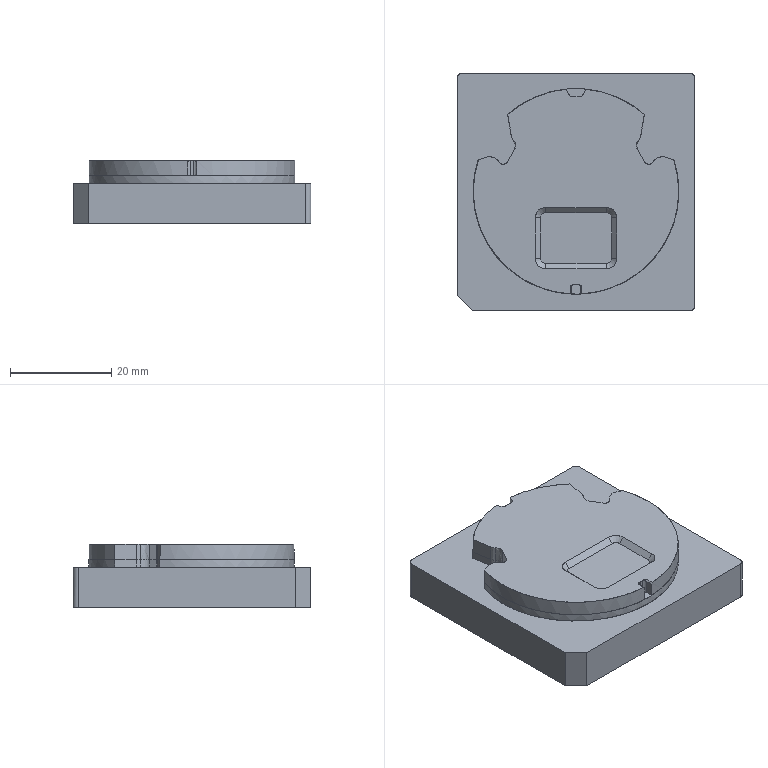NC program | PowerMill | posted with a generic post | part box 47 x 47 x 12.511 mm
Lines 1 to 1030 of 154620:
%
O0001
N104 ( POWERMILL CB  : 2026004.0)
N105 ( POST VER      : 2026.0.0.5161)
N106 ( OPTION FILE   : FANUC)
N107 ( OUTPUT WORKPLANE : WORLD)
N108 (  )
N109 ( TOOL LIST )
N110 (---------------------------------------)
N111 ( NO. | ID        | DIA.| TIP RAD|LENGTH)
N112 (---------------------------------------)
N113 (    1|D10C_1_1   |10.0 |  0.0   |67.96 )
N114 (   15|D3C_1_1    | 3.0 |  0.0   |59.56 )
N115 (   27|D1C_2_1    | 1.0 |  0.0   |59.56 )
N116 (    3|D10_1_1    |10.0 |  0.0   |67.68 )
N117 (   14|D4_2_1     | 4.0 |  0.0   |59.56 )
N118 (   12|D2_3       | 2.0 |  0.0   | 57.0 )
N119 (   12|D2_4_1     | 2.0 |  0.0   |59.56 )
N120 (    8|D1_2_1     | 1.0 |  0.0   |58.28 )
N121 (   13|TEXT_D4_1_1| 4.0 |  0.3   | 60.0 )
N122 (---------------------------------------)
N123 (  )
N124 ( NUMBER OF TOOLPATHS: 15.0 )
N125 ( ESTIMATED PROGRAM DURATION: 0 HOURS 20 MIN 55 SEC)
N126 (  )
N127 G00 G21 G80 G40 G17
N128 G90
N129 G54
N130 G53 Z0.0
N131 (---------------)
N132 ( START TOOLPATH : 粗公开粗01-扫面平行-D10C )
N133 (---------------)
N134 ( TOOL NO.    :1 )
N135 ( TOOL TYPE   : ENDMILL)
N136 ( TOOL ID     : D10C_1_1)
N137 ( TOOL DIA    : 10.0 LENGTH 67.96)
N138 T1
N139 M6
N140 S8000 M03
N141 G00 G90 X0.0 Y0.0
N142 G43 Z10.2 H1
N143
N144 G05 P10000 R4
N145 X31.15 Y26.15
N146 Z1.001
N147 G01 Z-0.199 F6000.0
N148 X26.15 F10000.0
N149 X-26.15
N150 Y20.3389
N151 X26.15
N152 Y14.5278
N153 X-26.15
N154 Y8.7167
N155 X26.15
N156 Y2.9056
N157 X-26.15
N158 Y-2.9056
N159 X26.15
N160 Y-8.7167
N161 X-26.15
N162 Y-14.5278
N163 X26.15
N164 Y-20.3389
N165 X-26.15
N166 Y-26.15
N167 X26.15
N168 X31.15
N169 G00 Z10.2
N170 G05 P0
N171 (---------------)
N172 ( END TOOLPATH : 粗公开粗01-扫面平行-D10C )
N173 (---------------)
N174 ( START TOOLPATH : 粗公开粗01-外形偏置-D10C )
N175 (---------------)
N176 G00 X-0.0005 Y0.117 Z9.8015
N177 G05 P10000 R4
N178 X33.241 Y4.78
N179 Z0.5591
N180 G01 Z-0.6409 F6000.0
N181 X32.7135 F10000.0
N182 G03 X27.966 Y0.0325 I0.0 J-4.7475
N183 G01 Y-21.3522
N184 X23.466
N185 X27.966
N186 Y-26.853
N187 G02 X26.966 Y-27.853 I-1.0 J0.0
N188 G01 X-26.967
N189 G02 X-27.967 Y-26.853 I0.0 J1.0
N190 G01 Y-21.3527
N191 X-23.467
N192 X-27.967
N193 Y21.0194
N194 X-23.467
N195 X-27.967
N196 Y27.087
N197 G02 X-26.967 Y28.087 I1.0 J0.0
N198 G01 X26.966
N199 G02 X27.966 Y27.087 I0.0 J-1.0
N200 G01 Y21.0207
N201 X23.466
N202 X27.966
N203 Y0.0325
N204 X25.4464 Y0.117
N205 X25.3946 Y-1.4299
N206 X25.3319 Y-2.2033
N207 X25.1511 Y-3.7501
N208 X24.8611 Y-5.297
N209 X24.4734 Y-6.8438
N210 X24.2389 Y-7.6173
N211 X23.6934 Y-9.1641
N212 X23.3727 Y-9.9375
N213 X22.6453 Y-11.4844
N214 X21.7804 Y-13.0313
N215 X20.882 Y-14.4266
N216 X20.1086 Y-15.4728
N217 X19.5854 Y-16.125
N218 X18.5617 Y-17.2865
N219 X17.0149 Y-18.8056
N220 X15.5941 Y-19.9921
N221 X14.5366 Y-20.7655
N222 X13.9212 Y-21.1835
N223 X12.3743 Y-22.1182
N224 X10.8275 Y-22.9082
N225 X9.2806 Y-23.5717
N226 X8.5072 Y-23.862
N227 X6.9603 Y-24.3596
N228 X5.9016 Y-24.6326
N229 X4.6401 Y-24.8983
N230 X3.0932 Y-25.1392
N231 X1.5464 Y-25.2797
N232 X0.7729 Y-25.3073
N233 X0.3875 Y-25.2817
N234 X0.0645 Y-25.2322
N235 X-0.0006 Y-25.2266
N236 X-0.0658 Y-25.2295
N237 X-0.7739 Y-25.3074
N238 X-1.5474 Y-25.2797
N239 X-3.0942 Y-25.1389
N240 X-3.8676 Y-25.0247
N241 X-5.4145 Y-24.7456
N242 X-6.9613 Y-24.3576
N243 X-8.5151 Y-23.8592
N244 X-9.2816 Y-23.5706
N245 X-10.8285 Y-22.9109
N246 X-12.3753 Y-22.1181
N247 X-13.9222 Y-21.183
N248 X-14.5366 Y-20.7655
N249 X-15.5945 Y-19.9921
N250 X-17.0159 Y-18.8048
N251 X-18.5627 Y-17.2897
N252 X-19.5864 Y-16.125
N253 X-20.1096 Y-15.4715
N254 X-20.883 Y-14.4252
N255 X-21.7821 Y-13.0312
N256 X-22.6452 Y-11.4844
N257 X-23.3727 Y-9.9375
N258 X-23.9767 Y-8.3978
N259 X-24.4734 Y-6.8438
N260 X-24.8612 Y-5.297
N261 X-25.1477 Y-3.7501
N262 X-25.247 Y-2.9767
N263 X-25.3957 Y-1.4299
N264 X-25.4454 Y0.117
N265 X-25.393 Y1.6639
N266 X-25.2544 Y3.2107
N267 X-25.0173 Y4.7576
N268 X-24.7501 Y6.0333
N269 X-24.2421 Y7.8513
N270 X-23.9767 Y8.5304
N271 X-23.4525 Y9.3981
N272 X-23.2033 Y9.7049
N273 X-22.7399 Y10.1715
N274 X-22.4299 Y10.423
N275 X-21.6564 Y10.9055
N276 X-20.883 Y11.2264
N277 X-19.5297 Y11.7184
N278 X-18.6231 Y11.9543
N279 G03 X-18.2566 Y12.525 I-0.1259 J0.4839
N280 G01 X-18.5627 Y14.2617
N281 X-18.6382 Y14.8121
N282 X-18.6486 Y15.5855
N283 X-18.5627 Y16.2623
N284 X-18.3098 Y17.1324
N285 X-17.9317 Y17.9058
N286 X-17.7893 Y18.1308
N287 X-17.3657 Y18.6792
N288 X-17.0159 Y19.0377
N289 X-15.5948 Y20.2261
N290 X-14.5342 Y20.9995
N291 X-13.1488 Y21.8993
N292 X-12.3753 Y22.3483
N293 X-10.8285 Y23.143
N294 X-9.2816 Y23.8111
N295 X-7.7348 Y24.3584
N296 X-5.9187 Y24.8666
N297 X-5.4145 Y24.9767
N298 X-3.8676 Y25.2608
N299 X-2.3208 Y25.458
N300 X-1.5474 Y25.4571
N301 X-0.7739 Y25.3458
N302 X-0.1601 Y25.155
N303 X-0.0143 Y25.1325
N304 X0.1317 Y25.1535
N305 X0.7729 Y25.3454
N306 X1.5464 Y25.457
N307 X2.3198 Y25.4581
N308 X3.0932 Y25.3642
N309 X4.6401 Y25.1288
N310 X5.9185 Y24.8666
N311 X7.7338 Y24.3587
N312 X9.2806 Y23.8113
N313 X10.8275 Y23.1432
N314 X11.9986 Y22.5464
N315 X13.1477 Y21.9
N316 X14.5343 Y20.9995
N317 X15.5948 Y20.2261
N318 X17.0149 Y19.0387
N319 X17.3659 Y18.6792
N320 X17.7883 Y18.1323
N321 X17.9296 Y17.9058
N322 X18.3098 Y17.1324
N323 X18.5428 Y16.359
N324 X18.6503 Y15.5855
N325 X18.6384 Y14.8121
N326 X18.5617 Y14.256
N327 X18.2557 Y12.5263
N328 G03 X18.6272 Y11.954 I0.4924 J-0.0872
N329 G01 X19.3352 Y11.7777
N330 X20.1086 Y11.5106
N331 X21.5803 Y10.945
N332 X22.4289 Y10.4238
N333 X22.7389 Y10.1715
N334 X23.2023 Y9.7055
N335 X23.4512 Y9.3981
N336 X23.9295 Y8.6247
N337 X24.2433 Y7.8513
N338 X24.6802 Y6.3044
N339 X25.0173 Y4.7576
N340 X25.2545 Y3.2107
N341 X25.3939 Y1.6639
N342 X25.4464 Y0.117
N343 X27.966 Y0.0325
N344 G00 Z3.2172
N345 G01 X33.241 Y4.78
N346 G00 Z0.1672
N347 G01 Z-1.0328 F6000.0
N348 X32.7135 F10000.0
N349 G03 X27.966 Y0.0325 I0.0 J-4.7475
N350 G01 Y-21.355
N351 X23.466
N352 X27.966
N353 Y-26.853
N354 G02 X26.966 Y-27.853 I-1.0 J0.0
N355 G01 X-26.967
N356 G02 X-27.967 Y-26.853 I0.0 J1.0
N357 G01 Y-21.3552
N358 X-23.467
N359 X-27.967
N360 Y0.1926
N361 X-25.4501 Y0.117
N362 X-25.4269 Y0.8904
N363 X-25.4072 Y1.2442
N364 X-25.393 Y1.6638
N365 X-25.3686 Y1.9356
N366 X-25.3406 Y2.4373
N367 X-25.2748 Y2.9825
N368 X-25.2544 Y3.2107
N369 X-25.2211 Y3.4282
N370 X-25.154 Y3.9841
N371 X-25.0702 Y4.4119
N372 X-25.0172 Y4.7575
N373 X-24.7929 Y5.8289
N374 X-24.7501 Y6.0474
N375 X-24.2472 Y7.8513
N376 X-23.9767 Y8.5393
N377 X-23.4572 Y9.3981
N378 X-23.2033 Y9.7116
N379 X-22.7456 Y10.1715
N380 X-22.4299 Y10.4296
N381 X-21.6564 Y10.9112
N382 X-20.883 Y11.2317
N383 X-19.5405 Y11.7184
N384 X-18.6268 Y11.9543
N385 G03 X-18.2594 Y12.5254 I-0.125 J0.4841
N386 G01 X-18.5627 Y14.2421
N387 X-18.6439 Y14.8121
N388 X-18.6541 Y15.5855
N389 X-18.5627 Y16.2815
N390 X-18.314 Y17.1324
N391 X-17.9361 Y17.9058
N392 X-17.7893 Y18.1376
N393 X-17.3707 Y18.6792
N394 X-17.0159 Y19.0425
N395 X-15.6004 Y20.2261
N396 X-15.3828 Y20.3806
N397 X-14.5342 Y20.9995
N398 X-14.2715 Y21.1701
N399 X-13.9222 Y21.4182
N400 X-13.4565 Y21.6994
N401 X-13.1487 Y21.8993
N402 X-12.542 Y22.2515
N403 X-12.3753 Y22.3522
N404 X-10.8285 Y23.1467
N405 X-9.2816 Y23.8147
N406 X-7.7348 Y24.3637
N407 X-5.9331 Y24.8666
N408 X-5.4145 Y24.9767
N409 X-3.8676 Y25.2665
N410 X-2.3208 Y25.4614
N411 X-1.5474 Y25.4642
N412 X-0.7739 Y25.3493
N413 X-0.1604 Y25.158
N414 X-0.0141 Y25.1353
N415 X0.1324 Y25.1565
N416 X0.7729 Y25.3491
N417 X1.5464 Y25.4641
N418 X2.3198 Y25.4615
N419 X3.067 Y25.3674
N420 X3.0932 Y25.3642
N421 X3.0978 Y25.3635
N422 X3.8666 Y25.2666
N423 X4.6401 Y25.1323
N424 X5.9329 Y24.8666
N425 X7.7338 Y24.3641
N426 X9.2806 Y23.8151
N427 X10.8275 Y23.1469
N428 X11.7671 Y22.6643
N429 X11.9986 Y22.5463
N430 X12.0177 Y22.5356
N431 X12.3743 Y22.3524
N432 X12.7984 Y22.0964
N433 X13.1477 Y21.8999
N434 X13.4617 Y21.696
N435 X13.9212 Y21.4186
N436 X14.2924 Y21.1565
N437 X14.5343 Y20.9995
N438 X15.1235 Y20.5698
N439 X15.468 Y20.3265
N440 X15.5479 Y20.2603
N441 X15.5948 Y20.226
N442 X16.2987 Y19.6375
N443 X17.0149 Y19.0434
N444 X17.3707 Y18.6792
N445 X17.7883 Y18.139
N446 X17.9361 Y17.9058
N447 X18.314 Y17.1324
N448 X18.5467 Y16.359
N449 X18.6541 Y15.5855
N450 X18.6439 Y14.8121
N451 X18.5617 Y14.2364
N452 X18.2577 Y12.5179
N453 X18.2503 Y12.4166
N454 X18.2634 Y12.3159
N455 G03 X18.6272 Y11.9539 I0.4847 J0.1233
N456 G01 X19.1135 Y11.8328
N457 X19.3352 Y11.7812
N458 X19.7098 Y11.6482
N459 X20.1086 Y11.5106
N460 X20.2388 Y11.4605
N461 X20.882 Y11.2322
N462 X21.5885 Y10.945
N463 X22.4289 Y10.4303
N464 X22.7455 Y10.1715
N465 X23.2023 Y9.7128
N466 X23.4572 Y9.3981
N467 X23.9349 Y8.6247
N468 X24.2472 Y7.8513
N469 X24.5537 Y6.7521
N470 X24.6802 Y6.3044
N471 X24.6859 Y6.2784
N472 X24.7491 Y6.0515
N473 X24.8721 Y5.4236
N474 X25.0173 Y4.7575
N475 X25.0701 Y4.4129
N476 X25.1541 Y3.9841
N477 X25.2205 Y3.4316
N478 X25.2544 Y3.2107
N479 X25.2763 Y2.968
N480 X25.3401 Y2.4373
N481 X25.3942 Y1.6639
N482 X25.4499 Y0.117
N483 X25.3983 Y-1.4299
N484 X25.335 Y-2.2033
N485 X25.1546 Y-3.7501
N486 X25.087 Y-4.0921
N487 X24.8611 Y-5.297
N488 X24.8022 Y-5.5317
N489 X24.7491 Y-5.8001
N490 X24.6033 Y-6.3255
N491 X24.4733 Y-6.8438
N492 X24.3069 Y-7.3927
N493 X24.2446 Y-7.6173
N494 X23.697 Y-9.1641
N495 X23.3727 Y-9.9375
N496 X22.6453 Y-11.4844
N497 X21.7851 Y-13.0313
N498 X20.882 Y-14.4325
N499 X20.1086 Y-15.4728
N500 X19.5907 Y-16.125
N501 X18.5617 Y-17.2917
N502 X17.0149 Y-18.8102
N503 X15.5996 Y-19.9921
N504 X15.3766 Y-20.1511
N505 X14.5366 Y-20.7655
N506 X14.0837 Y-21.073
N507 X13.9212 Y-21.1889
N508 X12.3743 Y-22.1222
N509 X11.8847 Y-22.3682
N510 X10.8274 Y-22.9081
N511 X10.7099 Y-22.9586
N512 X10.4567 Y-23.0858
N513 X9.8115 Y-23.3439
N514 X9.2806 Y-23.5716
N515 X8.6587 Y-23.8051
N516 X8.5072 Y-23.8657
N517 X6.9603 Y-24.3631
N518 X5.9017 Y-24.6326
N519 X4.6401 Y-24.901
N520 X3.0932 Y-25.1452
N521 X1.5464 Y-25.28
N522 X0.7729 Y-25.311
N523 X0.5696 Y-25.2937
N524 X0.3875 Y-25.2816
N525 X0.3385 Y-25.2741
N526 X0.1945 Y-25.2619
N527 X0.0656 Y-25.241
N528 X-0.0001 Y-25.2348
N529 X-0.066 Y-25.2373
N530 X-0.7739 Y-25.311
N531 X-1.5474 Y-25.28
N532 X-3.0942 Y-25.145
N533 X-3.8676 Y-25.0275
N534 X-5.4145 Y-24.7479
N535 X-6.9613 Y-24.363
N536 X-8.5262 Y-23.8592
N537 X-9.2816 Y-23.5731
N538 X-10.4568 Y-23.0858
N539 X-10.6733 Y-22.977
N540 X-10.8285 Y-22.9109
N541 X-11.9654 Y-22.3282
N542 X-12.3753 Y-22.1223
N543 X-13.9222 Y-21.188
N544 X-14.0965 Y-21.0645
N545 X-14.5366 Y-20.7655
N546 X-15.1045 Y-20.3503
N547 X-15.469 Y-20.092
N548 X-15.5528 Y-20.0226
N549 X-15.5945 Y-19.992
N550 X-16.2599 Y-19.4362
N551 X-17.0159 Y-18.8094
N552 X-18.5627 Y-17.2944
N553 X-19.5909 Y-16.125
N554 X-20.1096 Y-15.4715
N555 X-20.883 Y-14.4311
N556 X-21.785 Y-13.0312
N557 X-22.6452 Y-11.4844
N558 X-23.0265 Y-10.711
N559 X-23.2349 Y-10.2304
N560 X-23.3727 Y-9.9375
N561 X-23.4743 Y-9.6786
N562 X-23.6974 Y-9.1641
N563 X-23.893 Y-8.6112
N564 X-23.9767 Y-8.3978
N565 X-24.0538 Y-8.1565
N566 X-24.2445 Y-7.6173
N567 X-24.4734 Y-6.8438
N568 X-24.865 Y-5.297
N569 X-25.1547 Y-3.7501
N570 X-25.25 Y-2.9767
N571 X-25.3995 Y-1.4299
N572 X-25.4501 Y0.117
N573 X-27.967 Y0.1926
N574 Y21.0248
N575 X-23.467
N576 X-27.967
N577 Y27.087
N578 G02 X-26.967 Y28.087 I1.0 J0.0
N579 G01 X26.966
N580 G02 X27.966 Y27.087 I0.0 J-1.0
N581 G01 Y21.0261
N582 X23.466
N583 X27.966
N584 Y0.0325
N585 G00 Z2.8253
N586 G01 X33.241 Y4.78
N587 G00 Z-0.2247
N588 G01 Z-1.4247 F6000.0
N589 X32.7135 F10000.0
N590 G03 X27.966 Y0.0325 I0.0 J-4.7475
N591 G01 Y-21.3576
N592 X23.466
N593 X27.966
N594 Y-26.853
N595 G02 X26.966 Y-27.853 I-1.0 J0.0
N596 G01 X-26.967
N597 G02 X-27.967 Y-26.853 I0.0 J1.0
N598 G01 Y-21.3577
N599 X-23.467
N600 X-27.967
N601 Y-0.1593
N602 X-25.4472 Y-0.0764
N603 X-25.4535 Y0.117
N604 X-25.4301 Y0.8904
N605 X-25.4021 Y1.3933
N606 X-25.3929 Y1.6638
N607 X-25.3773 Y1.8383
N608 X-25.3439 Y2.4373
N609 X-25.2645 Y3.0976
N610 X-25.2543 Y3.2107
N611 X-25.2382 Y3.3158
N612 X-25.1578 Y3.9841
N613 X-25.057 Y4.498
N614 X-25.0172 Y4.7575
N615 X-24.8395 Y5.6063
N616 X-24.7501 Y6.0614
N617 X-24.2508 Y7.8513
N618 X-23.9767 Y8.5476
N619 X-23.462 Y9.3981
N620 X-23.2033 Y9.7174
N621 X-22.7513 Y10.1715
N622 X-22.4299 Y10.4343
N623 X-21.6564 Y10.9153
N624 X-20.883 Y11.2355
N625 X-19.5513 Y11.7184
N626 X-18.6309 Y11.9567
N627 G03 X-18.2639 Y12.5276 I-0.1254 J0.484
N628 G01 X-18.5627 Y14.2224
N629 X-18.6475 Y14.8121
N630 X-18.6579 Y15.5855
N631 X-18.5627 Y16.3008
N632 X-18.3182 Y17.1324
N633 X-17.9406 Y17.9058
N634 X-17.7893 Y18.1444
N635 X-17.3756 Y18.6792
N636 X-17.0159 Y19.0472
N637 X-15.6059 Y20.2261
N638 X-15.1707 Y20.5352
N639 X-14.5342 Y20.9994
N640 X-14.3372 Y21.1273
N641 X-13.9222 Y21.4222
N642 X-13.3698 Y21.7556
N643 X-13.1487 Y21.8992
N644 X-12.7101 Y22.1539
N645 X-12.3753 Y22.356
N646 X-10.8285 Y23.1504
N647 X-9.2816 Y23.8184
N648 X-7.7348 Y24.3673
N649 X-6.1879 Y24.803
N650 X-6.0423 Y24.8361
N651 X-5.933 Y24.8666
N652 X-5.5496 Y24.948
N653 X-5.4145 Y24.9787
N654 X-3.8676 Y25.2699
N655 X-2.3208 Y25.4649
N656 X-1.5474 Y25.4674
N657 X-0.7739 Y25.3522
N658 X-0.1605 Y25.1607
N659 X-0.0141 Y25.138
N660 X0.1326 Y25.1592
N661 X0.7729 Y25.352
N662 X1.5464 Y25.4673
N663 X2.3198 Y25.4649
N664 X3.8666 Y25.27
N665 X4.6401 Y25.1357
N666 X5.9473 Y24.8666
N667 X7.7338 Y24.3677
N668 X9.2806 Y23.8187
N669 X10.8275 Y23.1507
N670 X12.3743 Y22.3563
N671 X12.894 Y22.0426
N672 X13.1477 Y21.8999
N673 X13.3754 Y21.752
N674 X13.9212 Y21.4225
N675 X14.3641 Y21.1099
N676 X14.5342 Y20.9994
N677 X14.9433 Y20.7011
N678 X15.468 Y20.3308
N679 X15.5912 Y20.2286
N680 X15.5948 Y20.226
N681 X15.6461 Y20.1831
N682 X17.0149 Y19.0481
N683 X17.3756 Y18.6792
N684 X17.7883 Y18.1458
N685 X17.9406 Y17.9058
N686 X18.3182 Y17.1324
N687 X18.5507 Y16.359
N688 X18.6579 Y15.5855
N689 X18.6475 Y14.8121
N690 X18.5617 Y14.2168
N691 X18.2616 Y12.5206
N692 G03 X18.41 Y12.0706 I0.4924 J-0.0871
N693 G01 X18.5113 Y11.9986
N694 X18.6272 Y11.9539
N695 X18.8902 Y11.8884
N696 X19.3352 Y11.7848
N697 X20.0902 Y11.5168
N698 X20.1086 Y11.5105
N699 X20.1145 Y11.5082
N700 X20.882 Y11.2359
N701 X21.5966 Y10.945
N702 X22.4289 Y10.435
N703 X22.7513 Y10.1715
N704 X23.2023 Y9.7186
N705 X23.462 Y9.3981
N706 X23.9389 Y8.6247
N707 X24.2508 Y7.8513
N708 X24.7491 Y6.0656
N709 X24.9025 Y5.2843
N710 X25.0172 Y4.7575
N711 X25.0581 Y4.4911
N712 X25.1576 Y3.9841
N713 X25.2367 Y3.3258
N714 X25.2544 Y3.2107
N715 X25.2658 Y3.0842
N716 X25.3435 Y2.4373
N717 X25.3968 Y1.6639
N718 X25.4533 Y0.117
N719 X25.4018 Y-1.4299
N720 X25.3385 Y-2.2033
N721 X25.1581 Y-3.7501
N722 X25.0278 Y-4.4075
N723 X24.861 Y-5.297
N724 X24.8155 Y-5.4786
N725 X24.7491 Y-5.8133
N726 X24.5688 Y-6.4627
N727 X24.4733 Y-6.8438
N728 X24.3507 Y-7.2483
N729 X24.2482 Y-7.6173
N730 X23.7007 Y-9.1641
N731 X23.5994 Y-9.3969
N732 X23.3727 Y-9.9375
N733 X23.2575 Y-10.1824
N734 X23.0275 Y-10.711
N735 X22.6466 Y-11.4844
N736 X21.7892 Y-13.0313
N737 X20.882 Y-14.4385
N738 X20.7067 Y-14.6682
N739 X20.1085 Y-15.4728
N740 X19.7079 Y-15.9773
N741 X19.5952 Y-16.125
N742 X18.5617 Y-17.2968
N743 X17.0149 Y-18.8148
N744 X15.6051 Y-19.9921
N745 X15.1562 Y-20.3122
N746 X14.5366 Y-20.7654
N747 X14.206 Y-20.9899
N748 X13.9212 Y-21.193
N749 X12.3743 Y-22.1261
N750 X11.3733 Y-22.6293
N751 X10.8274 Y-22.9081
N752 X10.7682 Y-22.9335
N753 X10.4652 Y-23.0858
N754 X9.6573 Y-23.41
N755 X9.2806 Y-23.5716
N756 X8.8778 Y-23.7228
N757 X8.5378 Y-23.8592
N758 X6.9603 Y-24.3667
N759 X5.9052 Y-24.6326
N760 X4.6401 Y-24.9045
N761 X3.0932 Y-25.1486
N762 X2.3198 Y-25.2213
N763 X1.9911 Y-25.2412
N764 X1.5463 Y-25.2799
N765 X0.9571 Y-25.3036
N766 X0.7729 Y-25.3147
N767 X0.1943 Y-25.2659
N768 X0.0652 Y-25.2451
N769 X-0.0001 Y-25.239
N770 X-0.0657 Y-25.2414
N771 X-0.7739 Y-25.3147
N772 X-1.5474 Y-25.282
N773 X-3.0942 Y-25.1485
N774 X-3.8676 Y-25.0296
N775 X-5.4145 Y-24.7501
N776 X-6.9613 Y-24.3666
N777 X-8.5373 Y-23.8592
N778 X-8.7275 Y-23.7829
N779 X-9.2816 Y-23.573
N780 X-10.1993 Y-23.1925
N781 X-10.4653 Y-23.0858
N782 X-10.7299 Y-22.9528
N783 X-10.8284 Y-22.9108
N784 X-11.5659 Y-22.5329
N785 X-12.3753 Y-22.1262
N786 X-13.9222 Y-21.1924
N787 X-14.2543 Y-20.9572
N788 X-14.5366 Y-20.7654
N789 X-14.8908 Y-20.5064
N790 X-15.469 Y-20.097
N791 X-17.0159 Y-18.8139
N792 X-18.5627 Y-17.2991
N793 X-19.5955 Y-16.125
N794 X-19.7242 Y-15.957
N795 X-20.1095 Y-15.4715
N796 X-20.5439 Y-14.8873
N797 X-20.7808 Y-14.5781
N798 X-20.831 Y-14.501
N799 X-20.883 Y-14.4311
N800 X-21.4318 Y-13.5793
N801 X-21.789 Y-13.0312
N802 X-22.2318 Y-12.2578
N803 X-22.4463 Y-11.8421
N804 X-22.6452 Y-11.4844
N805 X-22.9581 Y-10.8496
N806 X-23.0296 Y-10.711
N807 X-23.2809 Y-10.1325
N808 X-23.3726 Y-9.9375
N809 X-23.4377 Y-9.7716
N810 X-23.7016 Y-9.1641
N811 X-23.9357 Y-8.5021
N812 X-23.9766 Y-8.3978
N813 X-24.0147 Y-8.2787
N814 X-24.2485 Y-7.6173
N815 X-24.4734 Y-6.8438
N816 X-24.868 Y-5.297
N817 X-25.1583 Y-3.7501
N818 X-25.2531 Y-2.9767
N819 X-25.4027 Y-1.4299
N820 X-25.4472 Y-0.0764
N821 X-27.967 Y-0.1593
N822 Y21.0301
N823 X-23.467
N824 X-27.967
N825 Y27.087
N826 G02 X-26.967 Y28.087 I1.0 J0.0
N827 G01 X26.966
N828 G02 X27.966 Y27.087 I0.0 J-1.0
N829 G01 Y21.0314
N830 X23.466
N831 X27.966
N832 Y0.0325
N833 G00 Z2.4334
N834 G01 X33.241 Y4.78
N835 G00 Z-0.6166
N836 G01 Z-1.8166 F6000.0
N837 X32.7135 F10000.0
N838 G03 X27.966 Y0.0325 I0.0 J-4.7475
N839 G01 Y-21.3602
N840 X23.466
N841 X27.966
N842 Y-26.853
N843 G02 X26.966 Y-27.853 I-1.0 J0.0
N844 G01 X-26.967
N845 G02 X-27.967 Y-26.853 I0.0 J1.0
N846 G01 Y-21.3602
N847 X-23.467
N848 X-27.967
N849 Y-0.1596
N850 X-25.4506 Y-0.0764
N851 X-25.457 Y0.117
N852 X-25.4333 Y0.8904
N853 X-25.3969 Y1.5431
N854 X-25.3929 Y1.6638
N855 X-25.3859 Y1.7414
N856 X-25.3472 Y2.4373
N857 X-25.2545 Y3.2086
N858 X-25.2543 Y3.2107
N859 X-25.254 Y3.2126
N860 X-25.1613 Y3.9841
N861 X-25.0451 Y4.5749
N862 X-25.0171 Y4.7575
N863 X-24.8879 Y5.375
N864 X-24.7501 Y6.0754
N865 X-24.2544 Y7.8513
N866 X-23.9767 Y8.5559
N867 X-23.4667 Y9.3981
N868 X-23.2033 Y9.7232
N869 X-22.7571 Y10.1715
N870 X-22.4299 Y10.439
N871 X-21.6564 Y10.9193
N872 X-20.883 Y11.2392
N873 X-19.5622 Y11.7184
N874 X-18.6339 Y11.9594
N875 G03 X-18.2672 Y12.5303 I-0.1257 J0.4839
N876 G01 X-18.5627 Y14.2028
N877 X-18.6511 Y14.8121
N878 X-18.6616 Y15.5855
N879 X-18.5627 Y16.32
N880 X-18.3224 Y17.1324
N881 X-17.9451 Y17.9058
N882 X-17.7893 Y18.1511
N883 X-17.3804 Y18.6792
N884 X-17.0159 Y19.0519
N885 X-15.6115 Y20.2261
N886 X-14.9585 Y20.6899
N887 X-14.5342 Y20.9994
N888 X-14.403 Y21.0846
N889 X-13.9222 Y21.4262
N890 X-13.2835 Y21.8116
N891 X-13.1487 Y21.8992
N892 X-12.8796 Y22.0554
N893 X-12.3753 Y22.3598
N894 X-10.8285 Y23.1541
N895 X-9.2816 Y23.822
N896 X-7.7348 Y24.371
N897 X-5.9618 Y24.8666
N898 X-5.4145 Y24.9821
N899 X-3.8676 Y25.2733
N900 X-2.3208 Y25.4683
N901 X-1.5474 Y25.4706
N902 X-0.7739 Y25.3552
N903 X-0.1607 Y25.1635
N904 X-0.0141 Y25.1407
N905 X0.1328 Y25.162
N906 X0.7729 Y25.3549
N907 X1.5464 Y25.4705
N908 X2.3198 Y25.4683
N909 X3.8666 Y25.2735
N910 X4.6401 Y25.1392
N911 X5.9617 Y24.8666
N912 X7.7338 Y24.3713
N913 X9.2806 Y23.8224
N914 X10.8275 Y23.1544
N915 X12.3743 Y22.3601
N916 X12.9908 Y21.9881
N917 X13.1477 Y21.8998
N918 X13.2878 Y21.8088
N919 X13.9212 Y21.4266
N920 X14.4377 Y21.0621
N921 X14.5342 Y20.9994
N922 X14.7643 Y20.8316
N923 X15.468 Y20.335
N924 X17.0149 Y19.0528
N925 X17.3804 Y18.6792
N926 X17.7883 Y18.1526
N927 X17.9451 Y17.9058
N928 X18.3224 Y17.1324
N929 X18.5547 Y16.359
N930 X18.6616 Y15.5855
N931 X18.6511 Y14.8121
N932 X18.6272 Y14.6714
N933 X18.5617 Y14.2168
N934 X18.2665 Y12.5486
N935 X18.2618 Y12.5206
N936 G03 X18.6011 Y11.9611 I0.4929 J-0.0837
N937 G01 X18.6141 Y11.9573
N938 X18.6272 Y11.9538
N939 X18.6652 Y11.9444
N940 X19.3352 Y11.7883
N941 X20.882 Y11.2395
N942 X21.6047 Y10.945
N943 X22.4289 Y10.4397
N944 X22.7571 Y10.1715
N945 X23.2023 Y9.7243
N946 X23.4667 Y9.3981
N947 X23.943 Y8.6247
N948 X24.2543 Y7.8513
N949 X24.7491 Y6.0797
N950 X24.9338 Y5.1403
N951 X25.0172 Y4.7575
N952 X25.0462 Y4.5683
N953 X25.161 Y3.9841
N954 X25.2529 Y3.22
N955 X25.2543 Y3.2107
N956 X25.2552 Y3.2004
N957 X25.347 Y2.4373
N958 X25.4003 Y1.6639
N959 X25.4567 Y0.117
N960 X25.4052 Y-1.4299
N961 X25.3419 Y-2.2033
N962 X25.1616 Y-3.7501
N963 X24.8701 Y-5.297
N964 X24.7491 Y-5.8265
N965 X24.5344 Y-6.5997
N966 X24.4732 Y-6.8438
N967 X24.3945 Y-7.1034
N968 X24.2518 Y-7.6173
N969 X23.7043 Y-9.1641
N970 X23.501 Y-9.6313
N971 X23.3726 Y-9.9375
N972 X23.3078 Y-10.0754
N973 X23.0312 Y-10.711
N974 X22.6504 Y-11.4844
N975 X21.7932 Y-13.0313
N976 X20.882 Y-14.4444
N977 X20.5317 Y-14.9036
N978 X20.1085 Y-15.4728
N979 X19.8252 Y-15.8296
N980 X19.5998 Y-16.125
N981 X18.5617 Y-17.302
N982 X17.0149 Y-18.8194
N983 X15.6106 Y-19.9921
N984 X14.9342 Y-20.4746
N985 X14.5365 Y-20.7654
N986 X14.326 Y-20.9083
N987 X13.9212 Y-21.1971
N988 X12.3743 Y-22.1301
N989 X10.838 Y-22.9026
N990 X10.8274 Y-22.908
N991 X10.8263 Y-22.9085
N992 X10.4737 Y-23.0858
N993 X9.5141 Y-23.4713
N994 X9.2806 Y-23.5715
N995 X9.04 Y-23.6619
N996 X8.5487 Y-23.8592
N997 X6.9603 Y-24.3703
N998 X5.9063 Y-24.6326
N999 X4.6401 Y-24.908
N1000 X3.0932 Y-25.1521
N1001 X2.3198 Y-25.2247
N1002 X1.8598 Y-25.2526
N1003 X1.5463 Y-25.2799
N1004 X1.1377 Y-25.2963
N1005 X0.7729 Y-25.3184
N1006 X0.1943 Y-25.27
N1007 X0.0649 Y-25.2492
N1008 X-0.0001 Y-25.2431
N1009 X-0.0654 Y-25.2456
N1010 X-0.7739 Y-25.3184
N1011 X-1.5474 Y-25.2853
N1012 X-3.0942 Y-25.1519
N1013 X-3.8676 Y-25.0318
N1014 X-5.4145 Y-24.7523
N1015 X-6.9613 Y-24.3702
N1016 X-8.5082 Y-23.8722
N1017 X-8.8041 Y-23.7539
N1018 X-9.2816 Y-23.573
N1019 X-9.9804 Y-23.2832
N1020 X-10.4738 Y-23.0858
N1021 X-10.7863 Y-22.9288
N1022 X-10.8284 Y-22.9108
N1023 X-11.1507 Y-22.7456
N1024 X-12.3753 Y-22.1301
N1025 X-13.9222 Y-21.1965
N1026 X-14.4002 Y-20.858
N1027 X-14.5365 Y-20.7654
N1028 X-14.7059 Y-20.6415
N1029 X-15.469 Y-20.1012
N1030 X-17.0159 Y-18.8185
N1031 X-18.5627 Y-17.3036
N1032 X-19.6 Y-16.125
N1033 X-19.8556 Y-15.7913
N1034 X-20.1095 Y-15.4715
N1035 X-20.3997 Y-15.0811
N1036 X-20.785 Y-14.5781
N1037 X-20.866 Y-14.4538
N1038 X-20.8829 Y-14.4311
N1039 X-21.0651 Y-14.1483
N1040 X-21.7931 Y-13.0312
N1041 X-22.235 Y-12.2578
N1042 X-22.4901 Y-11.7631
N1043 X-22.6452 Y-11.4844
N1044 X-22.8895 Y-10.9886
N1045 X-23.0327 Y-10.711
N1046 X-23.3244 Y-10.04
N1047 X-23.3726 Y-9.9375
N1048 X-23.4064 Y-9.8514
N1049 X-23.7051 Y-9.1641
N1050 X-23.9721 Y-8.4092
N1051 X-23.9766 Y-8.3977
N1052 X-23.9807 Y-8.3848
N1053 X-24.2521 Y-7.6173
N1054 X-24.4753 Y-6.8438
N1055 X-24.8711 Y-5.297
N1056 X-25.1617 Y-3.7501
N1057 X-25.2562 Y-2.9767
N1058 X-25.4058 Y-1.4299
N1059 X-25.4506 Y-0.0764
N1060 X-27.967 Y-0.1596
N1061 Y21.0354
N1062 X-23.467
N1063 X-27.967
N1064 Y27.087
N1065 G02 X-26.967 Y28.087 I1.0 J0.0
N1066 G01 X26.966
N1067 G02 X27.966 Y27.087 I0.0 J-1.0
N1068 G01 Y21.0367
N1069 X23.466
N1070 X27.966
N1071 Y0.0325
N1072 G00 Z2.0415
N1073 G01 X33.241 Y4.78
N1074 G00 Z-1.0085
N1075 G01 Z-2.2085 F6000.0
N1076 X32.7135 F10000.0
N1077 G03 X27.966 Y0.0325 I0.0 J-4.7475
N1078 G01 Y-21.3627
N1079 X23.466
N1080 X27.966
N1081 Y-26.853
N1082 G02 X26.966 Y-27.853 I-1.0 J0.0
N1083 G01 X-26.967
N1084 G02 X-27.967 Y-26.853 I0.0 J1.0
N1085 G01 Y-21.3626
N1086 X-23.467
N1087 X-27.967
N1088 Y0.1945
N1089 X-25.4604 Y0.117
N1090 X-25.4365 Y0.8904
N1091 X-25.3504 Y2.4373
N1092 X-25.1647 Y3.9841
N1093 X-25.0335 Y4.6507
N1094 X-25.0171 Y4.7575
N1095 X-24.9389 Y5.1309
N1096 X-24.7501 Y6.0895
N1097 X-24.258 Y7.8513
N1098 X-23.9767 Y8.5643
N1099 X-23.4714 Y9.3981
N1100 X-23.2033 Y9.7289
N1101 X-22.7628 Y10.1715
N1102 X-22.4299 Y10.4437
N1103 X-21.6564 Y10.9233
N1104 X-20.883 Y11.2428
N1105 X-19.573 Y11.7184
N1106 X-18.6349 Y11.9626
N1107 G03 X-18.2678 Y12.53 I-0.1259 J0.4838
N1108 G01 X-18.2853 Y12.6327
N1109 X-18.5627 Y14.2028
N1110 X-18.6295 Y14.6638
N1111 X-18.6547 Y14.8121
N1112 X-18.6654 Y15.5855
N1113 X-18.5627 Y16.3393
N1114 X-18.3266 Y17.1324
N1115 X-17.9495 Y17.9058
N1116 X-17.7893 Y18.1579
N1117 X-17.3852 Y18.6792
N1118 X-17.0159 Y19.0566
N1119 X-15.617 Y20.2261
N1120 X-14.7461 Y20.8447
N1121 X-14.5341 Y20.9994
N1122 X-14.4687 Y21.0419
N1123 X-13.9222 Y21.4301
N1124 X-13.1976 Y21.8674
N1125 X-13.1486 Y21.8992
N1126 X-13.0504 Y21.9562
N1127 X-12.3753 Y22.3636